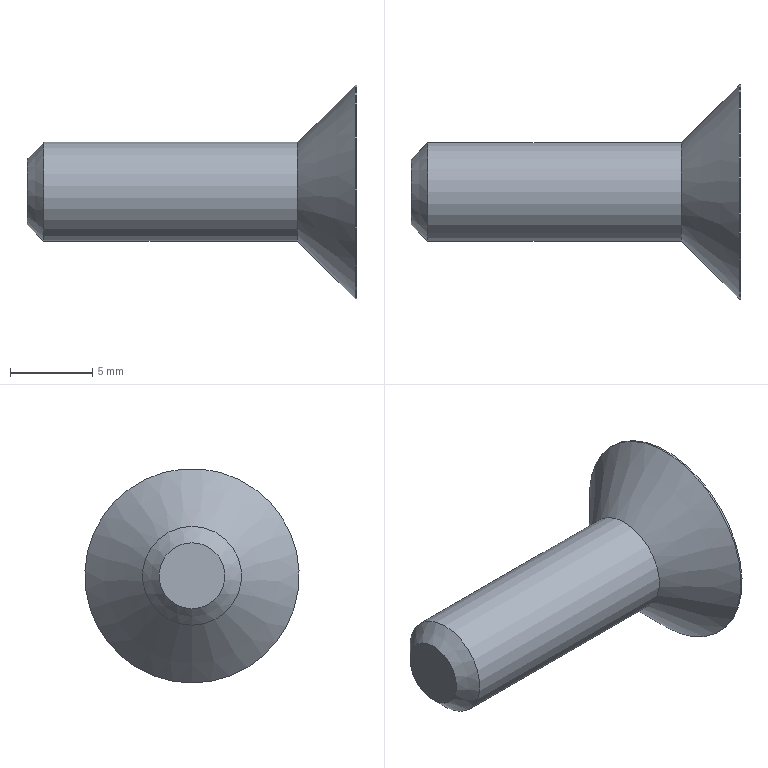Part | NX | features 5003_341_C-SFB6-20 2 | 1 solid | 13 faces | box 20 x 13 x 13 mm | volume 701.58 mm3 | plane 9 | cylinder 2 | cone 2 | commonest cylinder face diameters 6 x1 13 x1
STEP:
#1=CARTESIAN_POINT('',(-188.775,-588.445,-79.));
#2=VERTEX_POINT('',#1);
#3=CARTESIAN_POINT('',(-188.775,-587.291,-77.));
#4=VERTEX_POINT('',#3);
#5=CARTESIAN_POINT('',(-188.775,-588.445,-79.));
#6=DIRECTION('',(0.,0.5,0.866));
#7=VECTOR('',#6,1000.);
#8=LINE('',#5,#7);
#9=EDGE_CURVE('',#2,#4,#8,.T.);
#10=ORIENTED_EDGE('',*,*,#9,.F.);
#11=CARTESIAN_POINT('',(-188.775,-590.755,-79.));
#12=VERTEX_POINT('',#11);
#13=CARTESIAN_POINT('',(-188.775,-590.755,-79.));
#14=DIRECTION('',(0.,1.,0.));
#15=VECTOR('',#14,1000.);
#16=LINE('',#13,#15);
#17=EDGE_CURVE('',#12,#2,#16,.T.);
#18=ORIENTED_EDGE('',*,*,#17,.F.);
#19=CARTESIAN_POINT('',(-188.775,-591.909,-77.));
#20=VERTEX_POINT('',#19);
#21=CARTESIAN_POINT('',(-188.775,-591.909,-77.));
#22=DIRECTION('',(0.,0.5,-0.866));
#23=VECTOR('',#22,1000.);
#24=LINE('',#21,#23);
#25=EDGE_CURVE('',#20,#12,#24,.T.);
#26=ORIENTED_EDGE('',*,*,#25,.F.);
#27=CARTESIAN_POINT('',(-188.775,-590.755,-75.));
#28=VERTEX_POINT('',#27);
#29=CARTESIAN_POINT('',(-188.775,-590.755,-75.));
#30=DIRECTION('',(0.,-0.5,-0.866));
#31=VECTOR('',#30,1000.);
#32=LINE('',#29,#31);
#33=EDGE_CURVE('',#28,#20,#32,.T.);
#34=ORIENTED_EDGE('',*,*,#33,.F.);
#35=CARTESIAN_POINT('',(-188.775,-588.445,-75.));
#36=VERTEX_POINT('',#35);
#37=CARTESIAN_POINT('',(-188.775,-588.445,-75.));
#38=DIRECTION('',(0.,-1.,0.));
#39=VECTOR('',#38,1000.);
#40=LINE('',#37,#39);
#41=EDGE_CURVE('',#36,#28,#40,.T.);
#42=ORIENTED_EDGE('',*,*,#41,.F.);
#43=CARTESIAN_POINT('',(-188.775,-587.291,-77.));
#44=DIRECTION('',(0.,-0.5,0.866));
#45=VECTOR('',#44,1000.);
#46=LINE('',#43,#45);
#47=EDGE_CURVE('',#4,#36,#46,.T.);
#48=ORIENTED_EDGE('',*,*,#47,.F.);
#49=EDGE_LOOP('',(#10,#18,#26,#34,#42,#48));
#50=FACE_BOUND('',#49,.T.);
#51=CARTESIAN_POINT('',(-188.775,-589.6,-83.5));
#52=VERTEX_POINT('',#51);
#53=CARTESIAN_POINT('',(-188.775,-589.6,-77.));
#54=DIRECTION('',(1.,0.,0.));
#55=DIRECTION('',(0.,0.,-1.));
#56=AXIS2_PLACEMENT_3D('',#53,#54,#55);
#57=CIRCLE('',#56,6.5);
#58=EDGE_CURVE('',#52,#52,#57,.T.);
#59=ORIENTED_EDGE('',*,*,#58,.T.);
#60=EDGE_LOOP('',(#59));
#61=FACE_BOUND('',#60,.T.);
#62=CARTESIAN_POINT('',(-188.775,-596.1,-77.));
#63=DIRECTION('',(1.,0.,0.));
#64=DIRECTION('',(0.,0.,-1.));
#65=AXIS2_PLACEMENT_3D('',#62,#63,#64);
#66=PLANE('',#65);
#67=ADVANCED_FACE('',(#50,#61),#66,.T.);
#68=CARTESIAN_POINT('',(-188.875,-589.6,-83.5));
#69=VERTEX_POINT('',#68);
#70=CARTESIAN_POINT('',(-188.875,-589.6,-77.));
#71=DIRECTION('',(1.,0.,0.));
#72=DIRECTION('',(0.,0.,-1.));
#73=AXIS2_PLACEMENT_3D('',#70,#71,#72);
#74=CIRCLE('',#73,6.5);
#75=EDGE_CURVE('',#69,#69,#74,.T.);
#76=ORIENTED_EDGE('',*,*,#75,.T.);
#77=EDGE_LOOP('',(#76));
#78=FACE_BOUND('',#77,.T.);
#79=ORIENTED_EDGE('',*,*,#58,.F.);
#80=EDGE_LOOP('',(#79));
#81=FACE_BOUND('',#80,.T.);
#82=CARTESIAN_POINT('',(-188.775,-589.6,-77.));
#83=DIRECTION('',(1.,0.,0.));
#84=DIRECTION('',(0.,0.,-1.));
#85=AXIS2_PLACEMENT_3D('',#82,#83,#84);
#86=CYLINDRICAL_SURFACE('',#85,6.5);
#87=ADVANCED_FACE('',(#78,#81),#86,.T.);
#88=CARTESIAN_POINT('',(-192.375,-589.6,-80.));
#89=VERTEX_POINT('',#88);
#90=CARTESIAN_POINT('',(-192.375,-589.6,-77.));
#91=DIRECTION('',(1.,0.,0.));
#92=DIRECTION('',(0.,0.,-1.));
#93=AXIS2_PLACEMENT_3D('',#90,#91,#92);
#94=CIRCLE('',#93,3.);
#95=EDGE_CURVE('',#89,#89,#94,.T.);
#96=ORIENTED_EDGE('',*,*,#95,.T.);
#97=EDGE_LOOP('',(#96));
#98=FACE_BOUND('',#97,.T.);
#99=ORIENTED_EDGE('',*,*,#75,.F.);
#100=EDGE_LOOP('',(#99));
#101=FACE_BOUND('',#100,.T.);
#102=CARTESIAN_POINT('',(-188.875,-589.6,-77.));
#103=DIRECTION('',(1.,0.,0.));
#104=DIRECTION('',(0.,0.,-1.));
#105=AXIS2_PLACEMENT_3D('',#102,#103,#104);
#106=CONICAL_SURFACE('',#105,6.5,0.7854);
#107=ADVANCED_FACE('',(#98,#101),#106,.T.);
#108=CARTESIAN_POINT('',(-207.775,-589.6,-80.));
#109=VERTEX_POINT('',#108);
#110=CARTESIAN_POINT('',(-207.775,-589.6,-77.));
#111=DIRECTION('',(1.,0.,0.));
#112=DIRECTION('',(0.,0.,-1.));
#113=AXIS2_PLACEMENT_3D('',#110,#111,#112);
#114=CIRCLE('',#113,3.);
#115=EDGE_CURVE('',#109,#109,#114,.T.);
#116=ORIENTED_EDGE('',*,*,#115,.T.);
#117=EDGE_LOOP('',(#116));
#118=FACE_BOUND('',#117,.T.);
#119=ORIENTED_EDGE('',*,*,#95,.F.);
#120=EDGE_LOOP('',(#119));
#121=FACE_BOUND('',#120,.T.);
#122=CARTESIAN_POINT('',(-188.775,-589.6,-77.));
#123=DIRECTION('',(1.,0.,0.));
#124=DIRECTION('',(0.,0.,-1.));
#125=AXIS2_PLACEMENT_3D('',#122,#123,#124);
#126=CYLINDRICAL_SURFACE('',#125,3.);
#127=ADVANCED_FACE('',(#118,#121),#126,.T.);
#128=CARTESIAN_POINT('',(-208.775,-589.6,-79.));
#129=VERTEX_POINT('',#128);
#130=CARTESIAN_POINT('',(-208.775,-589.6,-77.));
#131=DIRECTION('',(1.,0.,0.));
#132=DIRECTION('',(0.,0.,-1.));
#133=AXIS2_PLACEMENT_3D('',#130,#131,#132);
#134=CIRCLE('',#133,2.);
#135=EDGE_CURVE('',#129,#129,#134,.T.);
#136=ORIENTED_EDGE('',*,*,#135,.T.);
#137=EDGE_LOOP('',(#136));
#138=FACE_BOUND('',#137,.T.);
#139=ORIENTED_EDGE('',*,*,#115,.F.);
#140=EDGE_LOOP('',(#139));
#141=FACE_BOUND('',#140,.T.);
#142=CARTESIAN_POINT('',(-207.775,-589.6,-77.));
#143=DIRECTION('',(1.,0.,0.));
#144=DIRECTION('',(0.,0.,-1.));
#145=AXIS2_PLACEMENT_3D('',#142,#143,#144);
#146=CONICAL_SURFACE('',#145,3.,0.7854);
#147=ADVANCED_FACE('',(#138,#141),#146,.T.);
#148=ORIENTED_EDGE('',*,*,#135,.F.);
#149=EDGE_LOOP('',(#148));
#150=FACE_BOUND('',#149,.T.);
#151=CARTESIAN_POINT('',(-208.775,-591.6,-77.));
#152=DIRECTION('',(-1.,0.,0.));
#153=DIRECTION('',(0.,0.,1.));
#154=AXIS2_PLACEMENT_3D('',#151,#152,#153);
#155=PLANE('',#154);
#156=ADVANCED_FACE('',(#150),#155,.T.);
#157=ORIENTED_EDGE('',*,*,#9,.T.);
#158=CARTESIAN_POINT('',(-190.675,-587.291,-77.));
#159=VERTEX_POINT('',#158);
#160=CARTESIAN_POINT('',(-190.675,-587.291,-77.));
#161=DIRECTION('',(1.,0.,0.));
#162=VECTOR('',#161,1000.);
#163=LINE('',#160,#162);
#164=EDGE_CURVE('',#159,#4,#163,.T.);
#165=ORIENTED_EDGE('',*,*,#164,.F.);
#166=CARTESIAN_POINT('',(-190.675,-588.445,-79.));
#167=VERTEX_POINT('',#166);
#168=CARTESIAN_POINT('',(-190.675,-588.445,-79.));
#169=DIRECTION('',(0.,0.5,0.866));
#170=VECTOR('',#169,1000.);
#171=LINE('',#168,#170);
#172=EDGE_CURVE('',#167,#159,#171,.T.);
#173=ORIENTED_EDGE('',*,*,#172,.F.);
#174=CARTESIAN_POINT('',(-190.675,-588.445,-79.));
#175=DIRECTION('',(1.,0.,0.));
#176=VECTOR('',#175,1000.);
#177=LINE('',#174,#176);
#178=EDGE_CURVE('',#167,#2,#177,.T.);
#179=ORIENTED_EDGE('',*,*,#178,.T.);
#180=EDGE_LOOP('',(#157,#165,#173,#179));
#181=FACE_BOUND('',#180,.T.);
#182=CARTESIAN_POINT('',(-190.675,-588.445,-79.));
#183=DIRECTION('',(0.,0.866,-0.5));
#184=DIRECTION('',(0.,-0.5,-0.866));
#185=AXIS2_PLACEMENT_3D('',#182,#183,#184);
#186=PLANE('',#185);
#187=ADVANCED_FACE('',(#181),#186,.F.);
#188=ORIENTED_EDGE('',*,*,#17,.T.);
#189=ORIENTED_EDGE('',*,*,#178,.F.);
#190=CARTESIAN_POINT('',(-190.675,-590.755,-79.));
#191=VERTEX_POINT('',#190);
#192=CARTESIAN_POINT('',(-190.675,-590.755,-79.));
#193=DIRECTION('',(0.,1.,0.));
#194=VECTOR('',#193,1000.);
#195=LINE('',#192,#194);
#196=EDGE_CURVE('',#191,#167,#195,.T.);
#197=ORIENTED_EDGE('',*,*,#196,.F.);
#198=CARTESIAN_POINT('',(-190.675,-590.755,-79.));
#199=DIRECTION('',(1.,0.,0.));
#200=VECTOR('',#199,1000.);
#201=LINE('',#198,#200);
#202=EDGE_CURVE('',#191,#12,#201,.T.);
#203=ORIENTED_EDGE('',*,*,#202,.T.);
#204=EDGE_LOOP('',(#188,#189,#197,#203));
#205=FACE_BOUND('',#204,.T.);
#206=CARTESIAN_POINT('',(-190.675,-590.755,-79.));
#207=DIRECTION('',(0.,0.,-1.));
#208=DIRECTION('',(-1.,0.,0.));
#209=AXIS2_PLACEMENT_3D('',#206,#207,#208);
#210=PLANE('',#209);
#211=ADVANCED_FACE('',(#205),#210,.F.);
#212=ORIENTED_EDGE('',*,*,#25,.T.);
#213=ORIENTED_EDGE('',*,*,#202,.F.);
#214=CARTESIAN_POINT('',(-190.675,-591.909,-77.));
#215=VERTEX_POINT('',#214);
#216=CARTESIAN_POINT('',(-190.675,-591.909,-77.));
#217=DIRECTION('',(0.,0.5,-0.866));
#218=VECTOR('',#217,1000.);
#219=LINE('',#216,#218);
#220=EDGE_CURVE('',#215,#191,#219,.T.);
#221=ORIENTED_EDGE('',*,*,#220,.F.);
#222=CARTESIAN_POINT('',(-190.675,-591.909,-77.));
#223=DIRECTION('',(1.,0.,0.));
#224=VECTOR('',#223,1000.);
#225=LINE('',#222,#224);
#226=EDGE_CURVE('',#215,#20,#225,.T.);
#227=ORIENTED_EDGE('',*,*,#226,.T.);
#228=EDGE_LOOP('',(#212,#213,#221,#227));
#229=FACE_BOUND('',#228,.T.);
#230=CARTESIAN_POINT('',(-190.675,-591.909,-77.));
#231=DIRECTION('',(0.,-0.866,-0.5));
#232=DIRECTION('',(0.,-0.5,0.866));
#233=AXIS2_PLACEMENT_3D('',#230,#231,#232);
#234=PLANE('',#233);
#235=ADVANCED_FACE('',(#229),#234,.F.);
#236=ORIENTED_EDGE('',*,*,#33,.T.);
#237=ORIENTED_EDGE('',*,*,#226,.F.);
#238=CARTESIAN_POINT('',(-190.675,-590.755,-75.));
#239=VERTEX_POINT('',#238);
#240=CARTESIAN_POINT('',(-190.675,-590.755,-75.));
#241=DIRECTION('',(0.,-0.5,-0.866));
#242=VECTOR('',#241,1000.);
#243=LINE('',#240,#242);
#244=EDGE_CURVE('',#239,#215,#243,.T.);
#245=ORIENTED_EDGE('',*,*,#244,.F.);
#246=CARTESIAN_POINT('',(-190.675,-590.755,-75.));
#247=DIRECTION('',(1.,0.,0.));
#248=VECTOR('',#247,1000.);
#249=LINE('',#246,#248);
#250=EDGE_CURVE('',#239,#28,#249,.T.);
#251=ORIENTED_EDGE('',*,*,#250,.T.);
#252=EDGE_LOOP('',(#236,#237,#245,#251));
#253=FACE_BOUND('',#252,.T.);
#254=CARTESIAN_POINT('',(-190.675,-590.755,-75.));
#255=DIRECTION('',(0.,-0.866,0.5));
#256=DIRECTION('',(0.,0.5,0.866));
#257=AXIS2_PLACEMENT_3D('',#254,#255,#256);
#258=PLANE('',#257);
#259=ADVANCED_FACE('',(#253),#258,.F.);
#260=ORIENTED_EDGE('',*,*,#41,.T.);
#261=ORIENTED_EDGE('',*,*,#250,.F.);
#262=CARTESIAN_POINT('',(-190.675,-588.445,-75.));
#263=VERTEX_POINT('',#262);
#264=CARTESIAN_POINT('',(-190.675,-588.445,-75.));
#265=DIRECTION('',(0.,-1.,0.));
#266=VECTOR('',#265,1000.);
#267=LINE('',#264,#266);
#268=EDGE_CURVE('',#263,#239,#267,.T.);
#269=ORIENTED_EDGE('',*,*,#268,.F.);
#270=CARTESIAN_POINT('',(-190.675,-588.445,-75.));
#271=DIRECTION('',(1.,0.,0.));
#272=VECTOR('',#271,1000.);
#273=LINE('',#270,#272);
#274=EDGE_CURVE('',#263,#36,#273,.T.);
#275=ORIENTED_EDGE('',*,*,#274,.T.);
#276=EDGE_LOOP('',(#260,#261,#269,#275));
#277=FACE_BOUND('',#276,.T.);
#278=CARTESIAN_POINT('',(-190.675,-588.445,-75.));
#279=DIRECTION('',(0.,0.,1.));
#280=DIRECTION('',(1.,0.,0.));
#281=AXIS2_PLACEMENT_3D('',#278,#279,#280);
#282=PLANE('',#281);
#283=ADVANCED_FACE('',(#277),#282,.F.);
#284=ORIENTED_EDGE('',*,*,#47,.T.);
#285=ORIENTED_EDGE('',*,*,#274,.F.);
#286=CARTESIAN_POINT('',(-190.675,-587.291,-77.));
#287=DIRECTION('',(0.,-0.5,0.866));
#288=VECTOR('',#287,1000.);
#289=LINE('',#286,#288);
#290=EDGE_CURVE('',#159,#263,#289,.T.);
#291=ORIENTED_EDGE('',*,*,#290,.F.);
#292=ORIENTED_EDGE('',*,*,#164,.T.);
#293=EDGE_LOOP('',(#284,#285,#291,#292));
#294=FACE_BOUND('',#293,.T.);
#295=CARTESIAN_POINT('',(-190.675,-587.291,-77.));
#296=DIRECTION('',(0.,0.866,0.5));
#297=DIRECTION('',(0.,0.5,-0.866));
#298=AXIS2_PLACEMENT_3D('',#295,#296,#297);
#299=PLANE('',#298);
#300=ADVANCED_FACE('',(#294),#299,.F.);
#301=ORIENTED_EDGE('',*,*,#172,.T.);
#302=ORIENTED_EDGE('',*,*,#290,.T.);
#303=ORIENTED_EDGE('',*,*,#268,.T.);
#304=ORIENTED_EDGE('',*,*,#244,.T.);
#305=ORIENTED_EDGE('',*,*,#220,.T.);
#306=ORIENTED_EDGE('',*,*,#196,.T.);
#307=EDGE_LOOP('',(#301,#302,#303,#304,#305,#306));
#308=FACE_BOUND('',#307,.T.);
#309=CARTESIAN_POINT('',(-190.675,-589.6,-77.));
#310=DIRECTION('',(1.,0.,0.));
#311=DIRECTION('',(0.,0.,-1.));
#312=AXIS2_PLACEMENT_3D('',#309,#310,#311);
#313=PLANE('',#312);
#314=ADVANCED_FACE('',(#308),#313,.T.);
#315=CLOSED_SHELL('',(#67,#87,#107,#127,#147,#156,#187,#211,#235,#259,#283,#300,#314));
#316=MANIFOLD_SOLID_BREP('',#315);
#317=(LENGTH_UNIT()NAMED_UNIT(*)SI_UNIT(.MILLI.,.METRE.));
#318=UNCERTAINTY_MEASURE_WITH_UNIT(LENGTH_MEASURE(0.00001),#317,'','');
#319=(NAMED_UNIT(*)PLANE_ANGLE_UNIT()SI_UNIT($,.RADIAN.));
#320=(NAMED_UNIT(*)SI_UNIT($,.STERADIAN.)SOLID_ANGLE_UNIT());
#321=(GEOMETRIC_REPRESENTATION_CONTEXT(3)GLOBAL_UNCERTAINTY_ASSIGNED_CONTEXT((#318))GLOBAL_UNIT_ASSIGNED_CONTEXT((#317,#319,#320))REPRESENTATION_CONTEXT('',''));
#322=ADVANCED_BREP_SHAPE_REPRESENTATION('',(#316),#321);